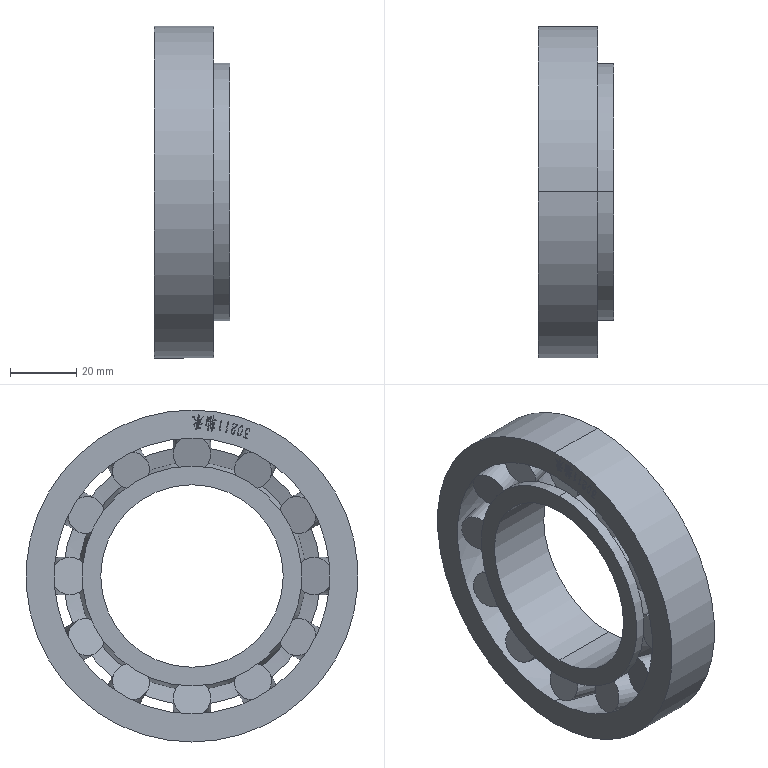Part | SolidWorks | features Revolution 5, CirPattern 1, ICE 1 | 17 solids | 448 faces | box 22.75 x 100 x 100 mm | volume 79449 mm3 | plane 291 | spline 111 | cylinder 38 | cone 8 | commonest cylinder face diameters 11.25 x30 55 x2 66.25 x2 77.5 x2 100 x2